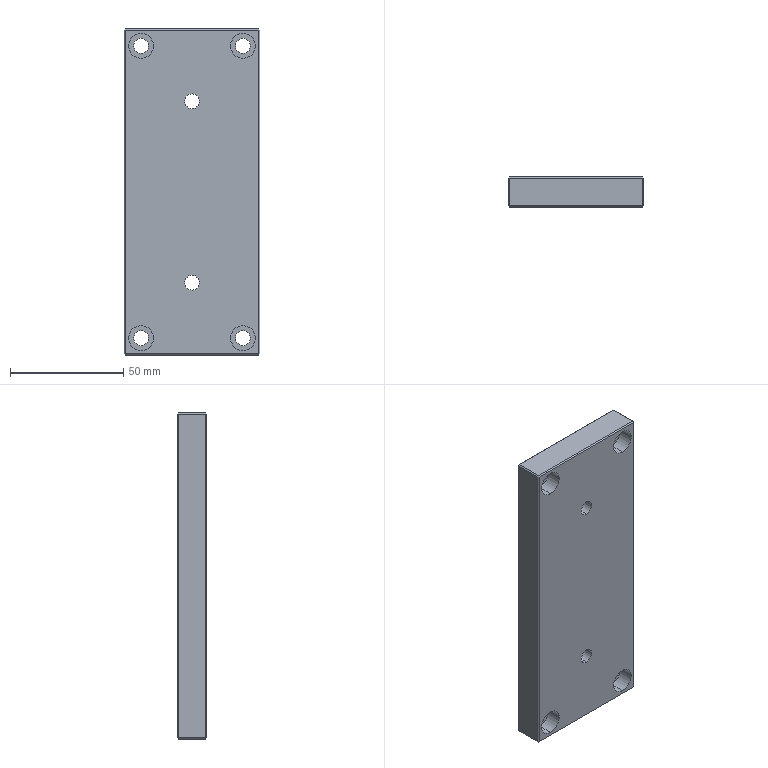Part | SolidWorks | features HoleWzd 2, Chamfer 1, Extrusion 1 | 1 solid | 56 faces | box 60 x 13 x 144 mm | volume 107062 mm3 | plane 32 | cylinder 24 | commonest cylinder face diameters 6.6 x12 11 x12
STEP:
#1=CARTESIAN_POINT('',(22.5,0.3,142.));
#2=VERTEX_POINT('',#1);
#3=CARTESIAN_POINT('',(22.5,0.3,131.));
#4=VERTEX_POINT('',#3);
#5=CARTESIAN_POINT('',(22.5,0.3,136.5));
#6=DIRECTION('',(0.,-1.,0.));
#7=DIRECTION('',(0.,0.,-1.));
#8=AXIS2_PLACEMENT_3D('',#5,#6,#7);
#9=CIRCLE('',#8,5.5);
#10=EDGE_CURVE('',#2,#4,#9,.T.);
#11=ORIENTED_EDGE('',*,*,#10,.F.);
#12=CARTESIAN_POINT('',(22.5,-6.5,142.));
#13=VERTEX_POINT('',#12);
#14=CARTESIAN_POINT('',(22.5,-6.5,142.));
#15=DIRECTION('',(0.,-1.,0.));
#16=VECTOR('',#15,1000.);
#17=LINE('',#14,#16);
#18=EDGE_CURVE('',#2,#13,#17,.T.);
#19=ORIENTED_EDGE('',*,*,#18,.T.);
#20=CARTESIAN_POINT('',(22.5,-6.5,131.));
#21=VERTEX_POINT('',#20);
#22=CARTESIAN_POINT('',(22.5,-6.5,136.5));
#23=DIRECTION('',(0.,-1.,0.));
#24=DIRECTION('',(0.,0.,-1.));
#25=AXIS2_PLACEMENT_3D('',#22,#23,#24);
#26=CIRCLE('',#25,5.5);
#27=EDGE_CURVE('',#13,#21,#26,.T.);
#28=ORIENTED_EDGE('',*,*,#27,.T.);
#29=CARTESIAN_POINT('',(22.5,-6.5,131.));
#30=DIRECTION('',(0.,-1.,0.));
#31=VECTOR('',#30,1000.);
#32=LINE('',#29,#31);
#33=EDGE_CURVE('',#4,#21,#32,.T.);
#34=ORIENTED_EDGE('',*,*,#33,.F.);
#35=EDGE_LOOP('',(#11,#19,#28,#34));
#36=FACE_OUTER_BOUND('',#35,.T.);
#37=CARTESIAN_POINT('',(22.5,-6.5,136.5));
#38=DIRECTION('',(0.,-1.,0.));
#39=DIRECTION('',(0.,0.,-1.));
#40=AXIS2_PLACEMENT_3D('',#37,#38,#39);
#41=CYLINDRICAL_SURFACE('',#40,5.5);
#42=ADVANCED_FACE('',(#36),#41,.F.);
#43=CARTESIAN_POINT('',(22.5,6.5,139.8));
#44=VERTEX_POINT('',#43);
#45=CARTESIAN_POINT('',(22.5,6.5,133.2));
#46=VERTEX_POINT('',#45);
#47=CARTESIAN_POINT('',(22.5,6.5,136.5));
#48=DIRECTION('',(0.,-1.,0.));
#49=DIRECTION('',(0.,0.,-1.));
#50=AXIS2_PLACEMENT_3D('',#47,#48,#49);
#51=CIRCLE('',#50,3.3);
#52=EDGE_CURVE('',#44,#46,#51,.T.);
#53=ORIENTED_EDGE('',*,*,#52,.F.);
#54=CARTESIAN_POINT('',(22.5,0.3,139.8));
#55=VERTEX_POINT('',#54);
#56=CARTESIAN_POINT('',(22.5,-6.5,139.8));
#57=DIRECTION('',(0.,-1.,0.));
#58=VECTOR('',#57,1000.);
#59=LINE('',#56,#58);
#60=EDGE_CURVE('',#44,#55,#59,.T.);
#61=ORIENTED_EDGE('',*,*,#60,.T.);
#62=CARTESIAN_POINT('',(22.5,0.3,133.2));
#63=VERTEX_POINT('',#62);
#64=CARTESIAN_POINT('',(22.5,0.3,136.5));
#65=DIRECTION('',(0.,-1.,0.));
#66=DIRECTION('',(0.,0.,-1.));
#67=AXIS2_PLACEMENT_3D('',#64,#65,#66);
#68=CIRCLE('',#67,3.3);
#69=EDGE_CURVE('',#55,#63,#68,.T.);
#70=ORIENTED_EDGE('',*,*,#69,.T.);
#71=CARTESIAN_POINT('',(22.5,-6.5,133.2));
#72=DIRECTION('',(0.,-1.,0.));
#73=VECTOR('',#72,1000.);
#74=LINE('',#71,#73);
#75=EDGE_CURVE('',#46,#63,#74,.T.);
#76=ORIENTED_EDGE('',*,*,#75,.F.);
#77=EDGE_LOOP('',(#53,#61,#70,#76));
#78=FACE_OUTER_BOUND('',#77,.T.);
#79=CARTESIAN_POINT('',(22.5,-6.5,136.5));
#80=DIRECTION('',(0.,-1.,0.));
#81=DIRECTION('',(0.,0.,-1.));
#82=AXIS2_PLACEMENT_3D('',#79,#80,#81);
#83=CYLINDRICAL_SURFACE('',#82,3.3);
#84=ADVANCED_FACE('',(#78),#83,.F.);
#85=CARTESIAN_POINT('',(-22.5,0.3,142.));
#86=VERTEX_POINT('',#85);
#87=CARTESIAN_POINT('',(-22.5,0.3,131.));
#88=VERTEX_POINT('',#87);
#89=CARTESIAN_POINT('',(-22.5,0.3,136.5));
#90=DIRECTION('',(0.,-1.,0.));
#91=DIRECTION('',(0.,0.,-1.));
#92=AXIS2_PLACEMENT_3D('',#89,#90,#91);
#93=CIRCLE('',#92,5.5);
#94=EDGE_CURVE('',#86,#88,#93,.T.);
#95=ORIENTED_EDGE('',*,*,#94,.F.);
#96=CARTESIAN_POINT('',(-22.5,-6.5,142.));
#97=VERTEX_POINT('',#96);
#98=CARTESIAN_POINT('',(-22.5,-6.5,142.));
#99=DIRECTION('',(0.,-1.,0.));
#100=VECTOR('',#99,1000.);
#101=LINE('',#98,#100);
#102=EDGE_CURVE('',#86,#97,#101,.T.);
#103=ORIENTED_EDGE('',*,*,#102,.T.);
#104=CARTESIAN_POINT('',(-22.5,-6.5,131.));
#105=VERTEX_POINT('',#104);
#106=CARTESIAN_POINT('',(-22.5,-6.5,136.5));
#107=DIRECTION('',(0.,-1.,0.));
#108=DIRECTION('',(0.,0.,-1.));
#109=AXIS2_PLACEMENT_3D('',#106,#107,#108);
#110=CIRCLE('',#109,5.5);
#111=EDGE_CURVE('',#97,#105,#110,.T.);
#112=ORIENTED_EDGE('',*,*,#111,.T.);
#113=CARTESIAN_POINT('',(-22.5,-6.5,131.));
#114=DIRECTION('',(0.,-1.,0.));
#115=VECTOR('',#114,1000.);
#116=LINE('',#113,#115);
#117=EDGE_CURVE('',#88,#105,#116,.T.);
#118=ORIENTED_EDGE('',*,*,#117,.F.);
#119=EDGE_LOOP('',(#95,#103,#112,#118));
#120=FACE_OUTER_BOUND('',#119,.T.);
#121=CARTESIAN_POINT('',(-22.5,-6.5,136.5));
#122=DIRECTION('',(0.,-1.,0.));
#123=DIRECTION('',(0.,0.,-1.));
#124=AXIS2_PLACEMENT_3D('',#121,#122,#123);
#125=CYLINDRICAL_SURFACE('',#124,5.5);
#126=ADVANCED_FACE('',(#120),#125,.F.);
#127=CARTESIAN_POINT('',(-22.5,6.5,139.8));
#128=VERTEX_POINT('',#127);
#129=CARTESIAN_POINT('',(-22.5,6.5,133.2));
#130=VERTEX_POINT('',#129);
#131=CARTESIAN_POINT('',(-22.5,6.5,136.5));
#132=DIRECTION('',(0.,-1.,0.));
#133=DIRECTION('',(0.,0.,-1.));
#134=AXIS2_PLACEMENT_3D('',#131,#132,#133);
#135=CIRCLE('',#134,3.3);
#136=EDGE_CURVE('',#128,#130,#135,.T.);
#137=ORIENTED_EDGE('',*,*,#136,.F.);
#138=CARTESIAN_POINT('',(-22.5,0.3,139.8));
#139=VERTEX_POINT('',#138);
#140=CARTESIAN_POINT('',(-22.5,-6.5,139.8));
#141=DIRECTION('',(0.,-1.,0.));
#142=VECTOR('',#141,1000.);
#143=LINE('',#140,#142);
#144=EDGE_CURVE('',#128,#139,#143,.T.);
#145=ORIENTED_EDGE('',*,*,#144,.T.);
#146=CARTESIAN_POINT('',(-22.5,0.3,133.2));
#147=VERTEX_POINT('',#146);
#148=CARTESIAN_POINT('',(-22.5,0.3,136.5));
#149=DIRECTION('',(0.,-1.,0.));
#150=DIRECTION('',(0.,0.,-1.));
#151=AXIS2_PLACEMENT_3D('',#148,#149,#150);
#152=CIRCLE('',#151,3.3);
#153=EDGE_CURVE('',#139,#147,#152,.T.);
#154=ORIENTED_EDGE('',*,*,#153,.T.);
#155=CARTESIAN_POINT('',(-22.5,-6.5,133.2));
#156=DIRECTION('',(0.,-1.,0.));
#157=VECTOR('',#156,1000.);
#158=LINE('',#155,#157);
#159=EDGE_CURVE('',#130,#147,#158,.T.);
#160=ORIENTED_EDGE('',*,*,#159,.F.);
#161=EDGE_LOOP('',(#137,#145,#154,#160));
#162=FACE_OUTER_BOUND('',#161,.T.);
#163=CARTESIAN_POINT('',(-22.5,-6.5,136.5));
#164=DIRECTION('',(0.,-1.,0.));
#165=DIRECTION('',(0.,0.,-1.));
#166=AXIS2_PLACEMENT_3D('',#163,#164,#165);
#167=CYLINDRICAL_SURFACE('',#166,3.3);
#168=ADVANCED_FACE('',(#162),#167,.F.);
#169=CARTESIAN_POINT('',(22.5,0.3,13.));
#170=VERTEX_POINT('',#169);
#171=CARTESIAN_POINT('',(22.5,0.3,2.));
#172=VERTEX_POINT('',#171);
#173=CARTESIAN_POINT('',(22.5,0.3,7.5));
#174=DIRECTION('',(0.,-1.,0.));
#175=DIRECTION('',(0.,0.,-1.));
#176=AXIS2_PLACEMENT_3D('',#173,#174,#175);
#177=CIRCLE('',#176,5.5);
#178=EDGE_CURVE('',#170,#172,#177,.T.);
#179=ORIENTED_EDGE('',*,*,#178,.F.);
#180=CARTESIAN_POINT('',(22.5,-6.5,13.));
#181=VERTEX_POINT('',#180);
#182=CARTESIAN_POINT('',(22.5,-6.5,13.));
#183=DIRECTION('',(0.,-1.,0.));
#184=VECTOR('',#183,1000.);
#185=LINE('',#182,#184);
#186=EDGE_CURVE('',#170,#181,#185,.T.);
#187=ORIENTED_EDGE('',*,*,#186,.T.);
#188=CARTESIAN_POINT('',(22.5,-6.5,2.));
#189=VERTEX_POINT('',#188);
#190=CARTESIAN_POINT('',(22.5,-6.5,7.5));
#191=DIRECTION('',(0.,-1.,0.));
#192=DIRECTION('',(0.,0.,-1.));
#193=AXIS2_PLACEMENT_3D('',#190,#191,#192);
#194=CIRCLE('',#193,5.5);
#195=EDGE_CURVE('',#181,#189,#194,.T.);
#196=ORIENTED_EDGE('',*,*,#195,.T.);
#197=CARTESIAN_POINT('',(22.5,-6.5,2.));
#198=DIRECTION('',(0.,-1.,0.));
#199=VECTOR('',#198,1000.);
#200=LINE('',#197,#199);
#201=EDGE_CURVE('',#172,#189,#200,.T.);
#202=ORIENTED_EDGE('',*,*,#201,.F.);
#203=EDGE_LOOP('',(#179,#187,#196,#202));
#204=FACE_OUTER_BOUND('',#203,.T.);
#205=CARTESIAN_POINT('',(22.5,-6.5,7.5));
#206=DIRECTION('',(0.,-1.,0.));
#207=DIRECTION('',(0.,0.,-1.));
#208=AXIS2_PLACEMENT_3D('',#205,#206,#207);
#209=CYLINDRICAL_SURFACE('',#208,5.5);
#210=ADVANCED_FACE('',(#204),#209,.F.);
#211=CARTESIAN_POINT('',(22.5,6.5,10.8));
#212=VERTEX_POINT('',#211);
#213=CARTESIAN_POINT('',(22.5,6.5,4.2));
#214=VERTEX_POINT('',#213);
#215=CARTESIAN_POINT('',(22.5,6.5,7.5));
#216=DIRECTION('',(0.,-1.,0.));
#217=DIRECTION('',(0.,0.,-1.));
#218=AXIS2_PLACEMENT_3D('',#215,#216,#217);
#219=CIRCLE('',#218,3.3);
#220=EDGE_CURVE('',#212,#214,#219,.T.);
#221=ORIENTED_EDGE('',*,*,#220,.F.);
#222=CARTESIAN_POINT('',(22.5,0.3,10.8));
#223=VERTEX_POINT('',#222);
#224=CARTESIAN_POINT('',(22.5,-6.5,10.8));
#225=DIRECTION('',(0.,-1.,0.));
#226=VECTOR('',#225,1000.);
#227=LINE('',#224,#226);
#228=EDGE_CURVE('',#212,#223,#227,.T.);
#229=ORIENTED_EDGE('',*,*,#228,.T.);
#230=CARTESIAN_POINT('',(22.5,0.3,4.2));
#231=VERTEX_POINT('',#230);
#232=CARTESIAN_POINT('',(22.5,0.3,7.5));
#233=DIRECTION('',(0.,-1.,0.));
#234=DIRECTION('',(0.,0.,-1.));
#235=AXIS2_PLACEMENT_3D('',#232,#233,#234);
#236=CIRCLE('',#235,3.3);
#237=EDGE_CURVE('',#223,#231,#236,.T.);
#238=ORIENTED_EDGE('',*,*,#237,.T.);
#239=CARTESIAN_POINT('',(22.5,-6.5,4.2));
#240=DIRECTION('',(0.,-1.,0.));
#241=VECTOR('',#240,1000.);
#242=LINE('',#239,#241);
#243=EDGE_CURVE('',#214,#231,#242,.T.);
#244=ORIENTED_EDGE('',*,*,#243,.F.);
#245=EDGE_LOOP('',(#221,#229,#238,#244));
#246=FACE_OUTER_BOUND('',#245,.T.);
#247=CARTESIAN_POINT('',(22.5,-6.5,7.5));
#248=DIRECTION('',(0.,-1.,0.));
#249=DIRECTION('',(0.,0.,-1.));
#250=AXIS2_PLACEMENT_3D('',#247,#248,#249);
#251=CYLINDRICAL_SURFACE('',#250,3.3);
#252=ADVANCED_FACE('',(#246),#251,.F.);
#253=CARTESIAN_POINT('',(-22.5,0.3,13.));
#254=VERTEX_POINT('',#253);
#255=CARTESIAN_POINT('',(-22.5,0.3,2.));
#256=VERTEX_POINT('',#255);
#257=CARTESIAN_POINT('',(-22.5,0.3,7.5));
#258=DIRECTION('',(0.,-1.,0.));
#259=DIRECTION('',(0.,0.,-1.));
#260=AXIS2_PLACEMENT_3D('',#257,#258,#259);
#261=CIRCLE('',#260,5.5);
#262=EDGE_CURVE('',#254,#256,#261,.T.);
#263=ORIENTED_EDGE('',*,*,#262,.F.);
#264=CARTESIAN_POINT('',(-22.5,-6.5,13.));
#265=VERTEX_POINT('',#264);
#266=CARTESIAN_POINT('',(-22.5,-6.5,13.));
#267=DIRECTION('',(0.,-1.,0.));
#268=VECTOR('',#267,1000.);
#269=LINE('',#266,#268);
#270=EDGE_CURVE('',#254,#265,#269,.T.);
#271=ORIENTED_EDGE('',*,*,#270,.T.);
#272=CARTESIAN_POINT('',(-22.5,-6.5,2.));
#273=VERTEX_POINT('',#272);
#274=CARTESIAN_POINT('',(-22.5,-6.5,7.5));
#275=DIRECTION('',(0.,-1.,0.));
#276=DIRECTION('',(0.,0.,-1.));
#277=AXIS2_PLACEMENT_3D('',#274,#275,#276);
#278=CIRCLE('',#277,5.5);
#279=EDGE_CURVE('',#265,#273,#278,.T.);
#280=ORIENTED_EDGE('',*,*,#279,.T.);
#281=CARTESIAN_POINT('',(-22.5,-6.5,2.));
#282=DIRECTION('',(0.,-1.,0.));
#283=VECTOR('',#282,1000.);
#284=LINE('',#281,#283);
#285=EDGE_CURVE('',#256,#273,#284,.T.);
#286=ORIENTED_EDGE('',*,*,#285,.F.);
#287=EDGE_LOOP('',(#263,#271,#280,#286));
#288=FACE_OUTER_BOUND('',#287,.T.);
#289=CARTESIAN_POINT('',(-22.5,-6.5,7.5));
#290=DIRECTION('',(0.,-1.,0.));
#291=DIRECTION('',(0.,0.,-1.));
#292=AXIS2_PLACEMENT_3D('',#289,#290,#291);
#293=CYLINDRICAL_SURFACE('',#292,5.5);
#294=ADVANCED_FACE('',(#288),#293,.F.);
#295=CARTESIAN_POINT('',(-22.5,6.5,10.8));
#296=VERTEX_POINT('',#295);
#297=CARTESIAN_POINT('',(-22.5,6.5,4.2));
#298=VERTEX_POINT('',#297);
#299=CARTESIAN_POINT('',(-22.5,6.5,7.5));
#300=DIRECTION('',(0.,-1.,0.));
#301=DIRECTION('',(0.,0.,-1.));
#302=AXIS2_PLACEMENT_3D('',#299,#300,#301);
#303=CIRCLE('',#302,3.3);
#304=EDGE_CURVE('',#296,#298,#303,.T.);
#305=ORIENTED_EDGE('',*,*,#304,.F.);
#306=CARTESIAN_POINT('',(-22.5,0.3,10.8));
#307=VERTEX_POINT('',#306);
#308=CARTESIAN_POINT('',(-22.5,-6.5,10.8));
#309=DIRECTION('',(0.,-1.,0.));
#310=VECTOR('',#309,1000.);
#311=LINE('',#308,#310);
#312=EDGE_CURVE('',#296,#307,#311,.T.);
#313=ORIENTED_EDGE('',*,*,#312,.T.);
#314=CARTESIAN_POINT('',(-22.5,0.3,4.2));
#315=VERTEX_POINT('',#314);
#316=CARTESIAN_POINT('',(-22.5,0.3,7.5));
#317=DIRECTION('',(0.,-1.,0.));
#318=DIRECTION('',(0.,0.,-1.));
#319=AXIS2_PLACEMENT_3D('',#316,#317,#318);
#320=CIRCLE('',#319,3.3);
#321=EDGE_CURVE('',#307,#315,#320,.T.);
#322=ORIENTED_EDGE('',*,*,#321,.T.);
#323=CARTESIAN_POINT('',(-22.5,-6.5,4.2));
#324=DIRECTION('',(0.,-1.,0.));
#325=VECTOR('',#324,1000.);
#326=LINE('',#323,#325);
#327=EDGE_CURVE('',#298,#315,#326,.T.);
#328=ORIENTED_EDGE('',*,*,#327,.F.);
#329=EDGE_LOOP('',(#305,#313,#322,#328));
#330=FACE_OUTER_BOUND('',#329,.T.);
#331=CARTESIAN_POINT('',(-22.5,-6.5,7.5));
#332=DIRECTION('',(0.,-1.,0.));
#333=DIRECTION('',(0.,0.,-1.));
#334=AXIS2_PLACEMENT_3D('',#331,#332,#333);
#335=CYLINDRICAL_SURFACE('',#334,3.3);
#336=ADVANCED_FACE('',(#330),#335,.F.);
#337=CARTESIAN_POINT('',(0.,-0.3,26.5));
#338=VERTEX_POINT('',#337);
#339=CARTESIAN_POINT('',(0.,-0.3,37.5));
#340=VERTEX_POINT('',#339);
#341=CARTESIAN_POINT('',(0.,-0.3,32.));
#342=DIRECTION('',(0.,1.,0.));
#343=DIRECTION('',(0.,0.,1.));
#344=AXIS2_PLACEMENT_3D('',#341,#342,#343);
#345=CIRCLE('',#344,5.5);
#346=EDGE_CURVE('',#338,#340,#345,.T.);
#347=ORIENTED_EDGE('',*,*,#346,.F.);
#348=CARTESIAN_POINT('',(0.,6.5,26.5));
#349=VERTEX_POINT('',#348);
#350=CARTESIAN_POINT('',(0.,6.5,26.5));
#351=DIRECTION('',(0.,1.,0.));
#352=VECTOR('',#351,1000.);
#353=LINE('',#350,#352);
#354=EDGE_CURVE('',#338,#349,#353,.T.);
#355=ORIENTED_EDGE('',*,*,#354,.T.);
#356=CARTESIAN_POINT('',(0.,6.5,37.5));
#357=VERTEX_POINT('',#356);
#358=CARTESIAN_POINT('',(0.,6.5,32.));
#359=DIRECTION('',(0.,1.,0.));
#360=DIRECTION('',(0.,0.,1.));
#361=AXIS2_PLACEMENT_3D('',#358,#359,#360);
#362=CIRCLE('',#361,5.5);
#363=EDGE_CURVE('',#349,#357,#362,.T.);
#364=ORIENTED_EDGE('',*,*,#363,.T.);
#365=CARTESIAN_POINT('',(0.,6.5,37.5));
#366=DIRECTION('',(0.,1.,0.));
#367=VECTOR('',#366,1000.);
#368=LINE('',#365,#367);
#369=EDGE_CURVE('',#340,#357,#368,.T.);
#370=ORIENTED_EDGE('',*,*,#369,.F.);
#371=EDGE_LOOP('',(#347,#355,#364,#370));
#372=FACE_OUTER_BOUND('',#371,.T.);
#373=CARTESIAN_POINT('',(0.,6.5,32.));
#374=DIRECTION('',(0.,1.,0.));
#375=DIRECTION('',(0.,0.,1.));
#376=AXIS2_PLACEMENT_3D('',#373,#374,#375);
#377=CYLINDRICAL_SURFACE('',#376,5.5);
#378=ADVANCED_FACE('',(#372),#377,.F.);
#379=CARTESIAN_POINT('',(0.,-6.5,28.7));
#380=VERTEX_POINT('',#379);
#381=CARTESIAN_POINT('',(0.,-6.5,35.3));
#382=VERTEX_POINT('',#381);
#383=CARTESIAN_POINT('',(0.,-6.5,32.));
#384=DIRECTION('',(0.,1.,0.));
#385=DIRECTION('',(0.,0.,1.));
#386=AXIS2_PLACEMENT_3D('',#383,#384,#385);
#387=CIRCLE('',#386,3.3);
#388=EDGE_CURVE('',#380,#382,#387,.T.);
#389=ORIENTED_EDGE('',*,*,#388,.F.);
#390=CARTESIAN_POINT('',(0.,-0.3,28.7));
#391=VERTEX_POINT('',#390);
#392=CARTESIAN_POINT('',(0.,6.5,28.7));
#393=DIRECTION('',(0.,1.,0.));
#394=VECTOR('',#393,1000.);
#395=LINE('',#392,#394);
#396=EDGE_CURVE('',#380,#391,#395,.T.);
#397=ORIENTED_EDGE('',*,*,#396,.T.);
#398=CARTESIAN_POINT('',(0.,-0.3,35.3));
#399=VERTEX_POINT('',#398);
#400=CARTESIAN_POINT('',(0.,-0.3,32.));
#401=DIRECTION('',(0.,1.,0.));
#402=DIRECTION('',(0.,0.,1.));
#403=AXIS2_PLACEMENT_3D('',#400,#401,#402);
#404=CIRCLE('',#403,3.3);
#405=EDGE_CURVE('',#391,#399,#404,.T.);
#406=ORIENTED_EDGE('',*,*,#405,.T.);
#407=CARTESIAN_POINT('',(0.,6.5,35.3));
#408=DIRECTION('',(0.,1.,0.));
#409=VECTOR('',#408,1000.);
#410=LINE('',#407,#409);
#411=EDGE_CURVE('',#382,#399,#410,.T.);
#412=ORIENTED_EDGE('',*,*,#411,.F.);
#413=EDGE_LOOP('',(#389,#397,#406,#412));
#414=FACE_OUTER_BOUND('',#413,.T.);
#415=CARTESIAN_POINT('',(0.,6.5,32.));
#416=DIRECTION('',(0.,1.,0.));
#417=DIRECTION('',(0.,0.,1.));
#418=AXIS2_PLACEMENT_3D('',#415,#416,#417);
#419=CYLINDRICAL_SURFACE('',#418,3.3);
#420=ADVANCED_FACE('',(#414),#419,.F.);
#421=CARTESIAN_POINT('',(0.,-0.3,106.5));
#422=VERTEX_POINT('',#421);
#423=CARTESIAN_POINT('',(0.,-0.3,117.5));
#424=VERTEX_POINT('',#423);
#425=CARTESIAN_POINT('',(0.,-0.3,112.));
#426=DIRECTION('',(0.,1.,0.));
#427=DIRECTION('',(0.,0.,1.));
#428=AXIS2_PLACEMENT_3D('',#425,#426,#427);
#429=CIRCLE('',#428,5.5);
#430=EDGE_CURVE('',#422,#424,#429,.T.);
#431=ORIENTED_EDGE('',*,*,#430,.F.);
#432=CARTESIAN_POINT('',(0.,6.5,106.5));
#433=VERTEX_POINT('',#432);
#434=CARTESIAN_POINT('',(0.,6.5,106.5));
#435=DIRECTION('',(0.,1.,0.));
#436=VECTOR('',#435,1000.);
#437=LINE('',#434,#436);
#438=EDGE_CURVE('',#422,#433,#437,.T.);
#439=ORIENTED_EDGE('',*,*,#438,.T.);
#440=CARTESIAN_POINT('',(0.,6.5,117.5));
#441=VERTEX_POINT('',#440);
#442=CARTESIAN_POINT('',(0.,6.5,112.));
#443=DIRECTION('',(0.,1.,0.));
#444=DIRECTION('',(0.,0.,1.));
#445=AXIS2_PLACEMENT_3D('',#442,#443,#444);
#446=CIRCLE('',#445,5.5);
#447=EDGE_CURVE('',#433,#441,#446,.T.);
#448=ORIENTED_EDGE('',*,*,#447,.T.);
#449=CARTESIAN_POINT('',(0.,6.5,117.5));
#450=DIRECTION('',(0.,1.,0.));
#451=VECTOR('',#450,1000.);
#452=LINE('',#449,#451);
#453=EDGE_CURVE('',#424,#441,#452,.T.);
#454=ORIENTED_EDGE('',*,*,#453,.F.);
#455=EDGE_LOOP('',(#431,#439,#448,#454));
#456=FACE_OUTER_BOUND('',#455,.T.);
#457=CARTESIAN_POINT('',(0.,6.5,112.));
#458=DIRECTION('',(0.,1.,0.));
#459=DIRECTION('',(0.,0.,1.));
#460=AXIS2_PLACEMENT_3D('',#457,#458,#459);
#461=CYLINDRICAL_SURFACE('',#460,5.5);
#462=ADVANCED_FACE('',(#456),#461,.F.);
#463=CARTESIAN_POINT('',(0.,-6.5,108.7));
#464=VERTEX_POINT('',#463);
#465=CARTESIAN_POINT('',(0.,-6.5,115.3));
#466=VERTEX_POINT('',#465);
#467=CARTESIAN_POINT('',(0.,-6.5,112.));
#468=DIRECTION('',(0.,1.,0.));
#469=DIRECTION('',(0.,0.,1.));
#470=AXIS2_PLACEMENT_3D('',#467,#468,#469);
#471=CIRCLE('',#470,3.3);
#472=EDGE_CURVE('',#464,#466,#471,.T.);
#473=ORIENTED_EDGE('',*,*,#472,.F.);
#474=CARTESIAN_POINT('',(0.,-0.3,108.7));
#475=VERTEX_POINT('',#474);
#476=CARTESIAN_POINT('',(0.,6.5,108.7));
#477=DIRECTION('',(0.,1.,0.));
#478=VECTOR('',#477,1000.);
#479=LINE('',#476,#478);
#480=EDGE_CURVE('',#464,#475,#479,.T.);
#481=ORIENTED_EDGE('',*,*,#480,.T.);
#482=CARTESIAN_POINT('',(0.,-0.3,115.3));
#483=VERTEX_POINT('',#482);
#484=CARTESIAN_POINT('',(0.,-0.3,112.));
#485=DIRECTION('',(0.,1.,0.));
#486=DIRECTION('',(0.,0.,1.));
#487=AXIS2_PLACEMENT_3D('',#484,#485,#486);
#488=CIRCLE('',#487,3.3);
#489=EDGE_CURVE('',#475,#483,#488,.T.);
#490=ORIENTED_EDGE('',*,*,#489,.T.);
#491=CARTESIAN_POINT('',(0.,6.5,115.3));
#492=DIRECTION('',(0.,1.,0.));
#493=VECTOR('',#492,1000.);
#494=LINE('',#491,#493);
#495=EDGE_CURVE('',#466,#483,#494,.T.);
#496=ORIENTED_EDGE('',*,*,#495,.F.);
#497=EDGE_LOOP('',(#473,#481,#490,#496));
#498=FACE_OUTER_BOUND('',#497,.T.);
#499=CARTESIAN_POINT('',(0.,6.5,112.));
#500=DIRECTION('',(0.,1.,0.));
#501=DIRECTION('',(0.,0.,1.));
#502=AXIS2_PLACEMENT_3D('',#499,#500,#501);
#503=CYLINDRICAL_SURFACE('',#502,3.3);
#504=ADVANCED_FACE('',(#498),#503,.F.);
#505=CARTESIAN_POINT('',(30.,6.,143.5));
#506=VERTEX_POINT('',#505);
#507=CARTESIAN_POINT('',(30.,-6.,143.5));
#508=VERTEX_POINT('',#507);
#509=CARTESIAN_POINT('',(30.,-6.5,143.5));
#510=DIRECTION('',(0.,-1.,0.));
#511=VECTOR('',#510,1000.);
#512=LINE('',#509,#511);
#513=EDGE_CURVE('',#506,#508,#512,.T.);
#514=ORIENTED_EDGE('',*,*,#513,.T.);
#515=CARTESIAN_POINT('',(30.,-6.,0.5));
#516=VERTEX_POINT('',#515);
#517=CARTESIAN_POINT('',(30.,-6.,144.));
#518=DIRECTION('',(0.,0.,-1.));
#519=VECTOR('',#518,1000.);
#520=LINE('',#517,#519);
#521=EDGE_CURVE('',#508,#516,#520,.T.);
#522=ORIENTED_EDGE('',*,*,#521,.T.);
#523=CARTESIAN_POINT('',(30.,6.,0.5));
#524=VERTEX_POINT('',#523);
#525=CARTESIAN_POINT('',(30.,6.5,0.5));
#526=DIRECTION('',(0.,1.,0.));
#527=VECTOR('',#526,1000.);
#528=LINE('',#525,#527);
#529=EDGE_CURVE('',#516,#524,#528,.T.);
#530=ORIENTED_EDGE('',*,*,#529,.T.);
#531=CARTESIAN_POINT('',(30.,6.,144.));
#532=DIRECTION('',(0.,0.,1.));
#533=VECTOR('',#532,1000.);
#534=LINE('',#531,#533);
#535=EDGE_CURVE('',#524,#506,#534,.T.);
#536=ORIENTED_EDGE('',*,*,#535,.T.);
#537=EDGE_LOOP('',(#514,#522,#530,#536));
#538=FACE_OUTER_BOUND('',#537,.T.);
#539=CARTESIAN_POINT('',(30.,6.5,144.));
#540=DIRECTION('',(-1.,0.,0.));
#541=DIRECTION('',(0.,0.,1.));
#542=AXIS2_PLACEMENT_3D('',#539,#540,#541);
#543=PLANE('',#542);
#544=ADVANCED_FACE('',(#538),#543,.F.);
#545=CARTESIAN_POINT('',(22.5,6.5,136.5));
#546=DIRECTION('',(0.,-1.,0.));
#547=DIRECTION('',(0.,0.,-1.));
#548=AXIS2_PLACEMENT_3D('',#545,#546,#547);
#549=CIRCLE('',#548,3.3);
#550=EDGE_CURVE('',#46,#44,#549,.T.);
#551=ORIENTED_EDGE('',*,*,#550,.T.);
#552=ORIENTED_EDGE('',*,*,#52,.T.);
#553=EDGE_LOOP('',(#551,#552));
#554=FACE_BOUND('',#553,.T.);
#555=CARTESIAN_POINT('',(-22.5,6.5,136.5));
#556=DIRECTION('',(0.,-1.,0.));
#557=DIRECTION('',(0.,0.,-1.));
#558=AXIS2_PLACEMENT_3D('',#555,#556,#557);
#559=CIRCLE('',#558,3.3);
#560=EDGE_CURVE('',#130,#128,#559,.T.);
#561=ORIENTED_EDGE('',*,*,#560,.T.);
#562=ORIENTED_EDGE('',*,*,#136,.T.);
#563=EDGE_LOOP('',(#561,#562));
#564=FACE_BOUND('',#563,.T.);
#565=CARTESIAN_POINT('',(22.5,6.5,7.5));
#566=DIRECTION('',(0.,-1.,0.));
#567=DIRECTION('',(0.,0.,-1.));
#568=AXIS2_PLACEMENT_3D('',#565,#566,#567);
#569=CIRCLE('',#568,3.3);
#570=EDGE_CURVE('',#214,#212,#569,.T.);
#571=ORIENTED_EDGE('',*,*,#570,.T.);
#572=ORIENTED_EDGE('',*,*,#220,.T.);
#573=EDGE_LOOP('',(#571,#572));
#574=FACE_BOUND('',#573,.T.);
#575=CARTESIAN_POINT('',(-22.5,6.5,7.5));
#576=DIRECTION('',(0.,-1.,0.));
#577=DIRECTION('',(0.,0.,-1.));
#578=AXIS2_PLACEMENT_3D('',#575,#576,#577);
#579=CIRCLE('',#578,3.3);
#580=EDGE_CURVE('',#298,#296,#579,.T.);
#581=ORIENTED_EDGE('',*,*,#580,.T.);
#582=ORIENTED_EDGE('',*,*,#304,.T.);
#583=EDGE_LOOP('',(#581,#582));
#584=FACE_BOUND('',#583,.T.);
#585=CARTESIAN_POINT('',(-29.5,6.5,0.5));
#586=VERTEX_POINT('',#585);
#587=CARTESIAN_POINT('',(-29.5,6.5,143.5));
#588=VERTEX_POINT('',#587);
#589=CARTESIAN_POINT('',(-29.5,6.5,144.));
#590=DIRECTION('',(0.,0.,1.));
#591=VECTOR('',#590,1000.);
#592=LINE('',#589,#591);
#593=EDGE_CURVE('',#586,#588,#592,.T.);
#594=ORIENTED_EDGE('',*,*,#593,.T.);
#595=CARTESIAN_POINT('',(29.5,6.5,143.5));
#596=VERTEX_POINT('',#595);
#597=CARTESIAN_POINT('',(30.,6.5,143.5));
#598=DIRECTION('',(1.,0.,0.));
#599=VECTOR('',#598,1000.);
#600=LINE('',#597,#599);
#601=EDGE_CURVE('',#588,#596,#600,.T.);
#602=ORIENTED_EDGE('',*,*,#601,.T.);
#603=CARTESIAN_POINT('',(29.5,6.5,0.5));
#604=VERTEX_POINT('',#603);
#605=CARTESIAN_POINT('',(29.5,6.5,144.));
#606=DIRECTION('',(0.,0.,-1.));
#607=VECTOR('',#606,1000.);
#608=LINE('',#605,#607);
#609=EDGE_CURVE('',#596,#604,#608,.T.);
#610=ORIENTED_EDGE('',*,*,#609,.T.);
#611=CARTESIAN_POINT('',(-30.,6.5,0.5));
#612=DIRECTION('',(-1.,0.,0.));
#613=VECTOR('',#612,1000.);
#614=LINE('',#611,#613);
#615=EDGE_CURVE('',#604,#586,#614,.T.);
#616=ORIENTED_EDGE('',*,*,#615,.T.);
#617=EDGE_LOOP('',(#594,#602,#610,#616));
#618=FACE_OUTER_BOUND('',#617,.T.);
#619=CARTESIAN_POINT('',(0.,6.5,32.));
#620=DIRECTION('',(0.,1.,0.));
#621=DIRECTION('',(0.,0.,1.));
#622=AXIS2_PLACEMENT_3D('',#619,#620,#621);
#623=CIRCLE('',#622,5.5);
#624=EDGE_CURVE('',#357,#349,#623,.T.);
#625=ORIENTED_EDGE('',*,*,#624,.F.);
#626=ORIENTED_EDGE('',*,*,#363,.F.);
#627=EDGE_LOOP('',(#625,#626));
#628=FACE_BOUND('',#627,.T.);
#629=CARTESIAN_POINT('',(0.,6.5,112.));
#630=DIRECTION('',(0.,1.,0.));
#631=DIRECTION('',(0.,0.,1.));
#632=AXIS2_PLACEMENT_3D('',#629,#630,#631);
#633=CIRCLE('',#632,5.5);
#634=EDGE_CURVE('',#441,#433,#633,.T.);
#635=ORIENTED_EDGE('',*,*,#634,.F.);
#636=ORIENTED_EDGE('',*,*,#447,.F.);
#637=EDGE_LOOP('',(#635,#636));
#638=FACE_BOUND('',#637,.T.);
#639=CARTESIAN_POINT('',(-30.,6.5,144.));
#640=DIRECTION('',(0.,-1.,0.));
#641=DIRECTION('',(0.,0.,-1.));
#642=AXIS2_PLACEMENT_3D('',#639,#640,#641);
#643=PLANE('',#642);
#644=ADVANCED_FACE('',(#554,#564,#574,#584,#618,#628,#638),#643,.F.);
#645=CARTESIAN_POINT('',(-30.,-6.,143.5));
#646=VERTEX_POINT('',#645);
#647=CARTESIAN_POINT('',(-30.,6.,143.5));
#648=VERTEX_POINT('',#647);
#649=CARTESIAN_POINT('',(-30.,6.5,143.5));
#650=DIRECTION('',(0.,1.,0.));
#651=VECTOR('',#650,1000.);
#652=LINE('',#649,#651);
#653=EDGE_CURVE('',#646,#648,#652,.T.);
#654=ORIENTED_EDGE('',*,*,#653,.T.);
#655=CARTESIAN_POINT('',(-30.,6.,0.5));
#656=VERTEX_POINT('',#655);
#657=CARTESIAN_POINT('',(-30.,6.,144.));
#658=DIRECTION('',(0.,0.,-1.));
#659=VECTOR('',#658,1000.);
#660=LINE('',#657,#659);
#661=EDGE_CURVE('',#648,#656,#660,.T.);
#662=ORIENTED_EDGE('',*,*,#661,.T.);
#663=CARTESIAN_POINT('',(-30.,-6.,0.5));
#664=VERTEX_POINT('',#663);
#665=CARTESIAN_POINT('',(-30.,6.5,0.5));
#666=DIRECTION('',(0.,-1.,0.));
#667=VECTOR('',#666,1000.);
#668=LINE('',#665,#667);
#669=EDGE_CURVE('',#656,#664,#668,.T.);
#670=ORIENTED_EDGE('',*,*,#669,.T.);
#671=CARTESIAN_POINT('',(-30.,-6.,144.));
#672=DIRECTION('',(0.,0.,1.));
#673=VECTOR('',#672,1000.);
#674=LINE('',#671,#673);
#675=EDGE_CURVE('',#664,#646,#674,.T.);
#676=ORIENTED_EDGE('',*,*,#675,.T.);
#677=EDGE_LOOP('',(#654,#662,#670,#676));
#678=FACE_OUTER_BOUND('',#677,.T.);
#679=CARTESIAN_POINT('',(-30.,6.5,144.));
#680=DIRECTION('',(1.,0.,0.));
#681=DIRECTION('',(0.,0.,-1.));
#682=AXIS2_PLACEMENT_3D('',#679,#680,#681);
#683=PLANE('',#682);
#684=ADVANCED_FACE('',(#678),#683,.F.);
#685=CARTESIAN_POINT('',(22.5,-6.5,136.5));
#686=DIRECTION('',(0.,-1.,0.));
#687=DIRECTION('',(0.,0.,-1.));
#688=AXIS2_PLACEMENT_3D('',#685,#686,#687);
#689=CIRCLE('',#688,5.5);
#690=EDGE_CURVE('',#21,#13,#689,.T.);
#691=ORIENTED_EDGE('',*,*,#690,.F.);
#692=ORIENTED_EDGE('',*,*,#27,.F.);
#693=EDGE_LOOP('',(#691,#692));
#694=FACE_BOUND('',#693,.T.);
#695=CARTESIAN_POINT('',(-22.5,-6.5,136.5));
#696=DIRECTION('',(0.,-1.,0.));
#697=DIRECTION('',(0.,0.,-1.));
#698=AXIS2_PLACEMENT_3D('',#695,#696,#697);
#699=CIRCLE('',#698,5.5);
#700=EDGE_CURVE('',#105,#97,#699,.T.);
#701=ORIENTED_EDGE('',*,*,#700,.F.);
#702=ORIENTED_EDGE('',*,*,#111,.F.);
#703=EDGE_LOOP('',(#701,#702));
#704=FACE_BOUND('',#703,.T.);
#705=CARTESIAN_POINT('',(22.5,-6.5,7.5));
#706=DIRECTION('',(0.,-1.,0.));
#707=DIRECTION('',(0.,0.,-1.));
#708=AXIS2_PLACEMENT_3D('',#705,#706,#707);
#709=CIRCLE('',#708,5.5);
#710=EDGE_CURVE('',#189,#181,#709,.T.);
#711=ORIENTED_EDGE('',*,*,#710,.F.);
#712=ORIENTED_EDGE('',*,*,#195,.F.);
#713=EDGE_LOOP('',(#711,#712));
#714=FACE_BOUND('',#713,.T.);
#715=CARTESIAN_POINT('',(-22.5,-6.5,7.5));
#716=DIRECTION('',(0.,-1.,0.));
#717=DIRECTION('',(0.,0.,-1.));
#718=AXIS2_PLACEMENT_3D('',#715,#716,#717);
#719=CIRCLE('',#718,5.5);
#720=EDGE_CURVE('',#273,#265,#719,.T.);
#721=ORIENTED_EDGE('',*,*,#720,.F.);
#722=ORIENTED_EDGE('',*,*,#279,.F.);
#723=EDGE_LOOP('',(#721,#722));
#724=FACE_BOUND('',#723,.T.);
#725=CARTESIAN_POINT('',(29.5,-6.5,0.5));
#726=VERTEX_POINT('',#725);
#727=CARTESIAN_POINT('',(29.5,-6.5,143.5));
#728=VERTEX_POINT('',#727);
#729=CARTESIAN_POINT('',(29.5,-6.5,144.));
#730=DIRECTION('',(0.,0.,1.));
#731=VECTOR('',#730,1000.);
#732=LINE('',#729,#731);
#733=EDGE_CURVE('',#726,#728,#732,.T.);
#734=ORIENTED_EDGE('',*,*,#733,.T.);
#735=CARTESIAN_POINT('',(-29.5,-6.5,143.5));
#736=VERTEX_POINT('',#735);
#737=CARTESIAN_POINT('',(-30.,-6.5,143.5));
#738=DIRECTION('',(-1.,0.,0.));
#739=VECTOR('',#738,1000.);
#740=LINE('',#737,#739);
#741=EDGE_CURVE('',#728,#736,#740,.T.);
#742=ORIENTED_EDGE('',*,*,#741,.T.);
#743=CARTESIAN_POINT('',(-29.5,-6.5,0.5));
#744=VERTEX_POINT('',#743);
#745=CARTESIAN_POINT('',(-29.5,-6.5,144.));
#746=DIRECTION('',(0.,0.,-1.));
#747=VECTOR('',#746,1000.);
#748=LINE('',#745,#747);
#749=EDGE_CURVE('',#736,#744,#748,.T.);
#750=ORIENTED_EDGE('',*,*,#749,.T.);
#751=CARTESIAN_POINT('',(-30.,-6.5,0.5));
#752=DIRECTION('',(1.,0.,0.));
#753=VECTOR('',#752,1000.);
#754=LINE('',#751,#753);
#755=EDGE_CURVE('',#744,#726,#754,.T.);
#756=ORIENTED_EDGE('',*,*,#755,.T.);
#757=EDGE_LOOP('',(#734,#742,#750,#756));
#758=FACE_OUTER_BOUND('',#757,.T.);
#759=CARTESIAN_POINT('',(0.,-6.5,32.));
#760=DIRECTION('',(0.,1.,0.));
#761=DIRECTION('',(0.,0.,1.));
#762=AXIS2_PLACEMENT_3D('',#759,#760,#761);
#763=CIRCLE('',#762,3.3);
#764=EDGE_CURVE('',#382,#380,#763,.T.);
#765=ORIENTED_EDGE('',*,*,#764,.T.);
#766=ORIENTED_EDGE('',*,*,#388,.T.);
#767=EDGE_LOOP('',(#765,#766));
#768=FACE_BOUND('',#767,.T.);
#769=CARTESIAN_POINT('',(0.,-6.5,112.));
#770=DIRECTION('',(0.,1.,0.));
#771=DIRECTION('',(0.,0.,1.));
#772=AXIS2_PLACEMENT_3D('',#769,#770,#771);
#773=CIRCLE('',#772,3.3);
#774=EDGE_CURVE('',#466,#464,#773,.T.);
#775=ORIENTED_EDGE('',*,*,#774,.T.);
#776=ORIENTED_EDGE('',*,*,#472,.T.);
#777=EDGE_LOOP('',(#775,#776));
#778=FACE_BOUND('',#777,.T.);
#779=CARTESIAN_POINT('',(-30.,-6.5,144.));
#780=DIRECTION('',(0.,1.,0.));
#781=DIRECTION('',(0.,0.,1.));
#782=AXIS2_PLACEMENT_3D('',#779,#780,#781);
#783=PLANE('',#782);
#784=ADVANCED_FACE('',(#694,#704,#714,#724,#758,#768,#778),#783,.F.);
#785=CARTESIAN_POINT('',(29.5,6.,144.));
#786=VERTEX_POINT('',#785);
#787=CARTESIAN_POINT('',(-29.5,6.,144.));
#788=VERTEX_POINT('',#787);
#789=CARTESIAN_POINT('',(-30.,6.,144.));
#790=DIRECTION('',(-1.,0.,0.));
#791=VECTOR('',#790,1000.);
#792=LINE('',#789,#791);
#793=EDGE_CURVE('',#786,#788,#792,.T.);
#794=ORIENTED_EDGE('',*,*,#793,.T.);
#795=CARTESIAN_POINT('',(-29.5,-6.,144.));
#796=VERTEX_POINT('',#795);
#797=CARTESIAN_POINT('',(-29.5,-6.5,144.));
#798=DIRECTION('',(0.,-1.,0.));
#799=VECTOR('',#798,1000.);
#800=LINE('',#797,#799);
#801=EDGE_CURVE('',#788,#796,#800,.T.);
#802=ORIENTED_EDGE('',*,*,#801,.T.);
#803=CARTESIAN_POINT('',(29.5,-6.,144.));
#804=VERTEX_POINT('',#803);
#805=CARTESIAN_POINT('',(30.,-6.,144.));
#806=DIRECTION('',(1.,0.,0.));
#807=VECTOR('',#806,1000.);
#808=LINE('',#805,#807);
#809=EDGE_CURVE('',#796,#804,#808,.T.);
#810=ORIENTED_EDGE('',*,*,#809,.T.);
#811=CARTESIAN_POINT('',(29.5,6.5,144.));
#812=DIRECTION('',(0.,1.,0.));
#813=VECTOR('',#812,1000.);
#814=LINE('',#811,#813);
#815=EDGE_CURVE('',#804,#786,#814,.T.);
#816=ORIENTED_EDGE('',*,*,#815,.T.);
#817=EDGE_LOOP('',(#794,#802,#810,#816));
#818=FACE_OUTER_BOUND('',#817,.T.);
#819=CARTESIAN_POINT('',(0.,0.,144.));
#820=DIRECTION('',(0.,0.,1.));
#821=DIRECTION('',(1.,0.,0.));
#822=AXIS2_PLACEMENT_3D('',#819,#820,#821);
#823=PLANE('',#822);
#824=ADVANCED_FACE('',(#818),#823,.T.);
#825=CARTESIAN_POINT('',(29.5,-6.,0.));
#826=VERTEX_POINT('',#825);
#827=CARTESIAN_POINT('',(-29.5,-6.,0.));
#828=VERTEX_POINT('',#827);
#829=CARTESIAN_POINT('',(0.,-6.,0.));
#830=DIRECTION('',(-1.,0.,0.));
#831=VECTOR('',#830,1000.);
#832=LINE('',#829,#831);
#833=EDGE_CURVE('',#826,#828,#832,.T.);
#834=ORIENTED_EDGE('',*,*,#833,.T.);
#835=CARTESIAN_POINT('',(-29.5,6.,0.));
#836=VERTEX_POINT('',#835);
#837=CARTESIAN_POINT('',(-29.5,0.,0.));
#838=DIRECTION('',(0.,1.,0.));
#839=VECTOR('',#838,1000.);
#840=LINE('',#837,#839);
#841=EDGE_CURVE('',#828,#836,#840,.T.);
#842=ORIENTED_EDGE('',*,*,#841,.T.);
#843=CARTESIAN_POINT('',(29.5,6.,0.));
#844=VERTEX_POINT('',#843);
#845=CARTESIAN_POINT('',(0.,6.,0.));
#846=DIRECTION('',(1.,0.,0.));
#847=VECTOR('',#846,1000.);
#848=LINE('',#845,#847);
#849=EDGE_CURVE('',#836,#844,#848,.T.);
#850=ORIENTED_EDGE('',*,*,#849,.T.);
#851=CARTESIAN_POINT('',(29.5,0.,0.));
#852=DIRECTION('',(0.,-1.,0.));
#853=VECTOR('',#852,1000.);
#854=LINE('',#851,#853);
#855=EDGE_CURVE('',#844,#826,#854,.T.);
#856=ORIENTED_EDGE('',*,*,#855,.T.);
#857=EDGE_LOOP('',(#834,#842,#850,#856));
#858=FACE_OUTER_BOUND('',#857,.T.);
#859=CARTESIAN_POINT('',(0.,0.,0.));
#860=DIRECTION('',(0.,0.,1.));
#861=DIRECTION('',(1.,0.,0.));
#862=AXIS2_PLACEMENT_3D('',#859,#860,#861);
#863=PLANE('',#862);
#864=ADVANCED_FACE('',(#858),#863,.F.);
#865=ORIENTED_EDGE('',*,*,#480,.F.);
#866=ORIENTED_EDGE('',*,*,#774,.F.);
#867=ORIENTED_EDGE('',*,*,#495,.T.);
#868=CARTESIAN_POINT('',(0.,-0.3,112.));
#869=DIRECTION('',(0.,1.,0.));
#870=DIRECTION('',(0.,0.,1.));
#871=AXIS2_PLACEMENT_3D('',#868,#869,#870);
#872=CIRCLE('',#871,3.3);
#873=EDGE_CURVE('',#483,#475,#872,.T.);
#874=ORIENTED_EDGE('',*,*,#873,.T.);
#875=EDGE_LOOP('',(#865,#866,#867,#874));
#876=FACE_OUTER_BOUND('',#875,.T.);
#877=CARTESIAN_POINT('',(0.,6.5,112.));
#878=DIRECTION('',(0.,1.,0.));
#879=DIRECTION('',(0.,0.,1.));
#880=AXIS2_PLACEMENT_3D('',#877,#878,#879);
#881=CYLINDRICAL_SURFACE('',#880,3.3);
#882=ADVANCED_FACE('',(#876),#881,.F.);
#883=ORIENTED_EDGE('',*,*,#873,.F.);
#884=ORIENTED_EDGE('',*,*,#489,.F.);
#885=EDGE_LOOP('',(#883,#884));
#886=FACE_BOUND('',#885,.T.);
#887=CARTESIAN_POINT('',(0.,-0.3,112.));
#888=DIRECTION('',(0.,1.,0.));
#889=DIRECTION('',(0.,0.,1.));
#890=AXIS2_PLACEMENT_3D('',#887,#888,#889);
#891=CIRCLE('',#890,5.5);
#892=EDGE_CURVE('',#424,#422,#891,.T.);
#893=ORIENTED_EDGE('',*,*,#892,.T.);
#894=ORIENTED_EDGE('',*,*,#430,.T.);
#895=EDGE_LOOP('',(#893,#894));
#896=FACE_OUTER_BOUND('',#895,.T.);
#897=CARTESIAN_POINT('',(3.3,-0.3,112.));
#898=DIRECTION('',(0.,-1.,0.));
#899=DIRECTION('',(0.,0.,-1.));
#900=AXIS2_PLACEMENT_3D('',#897,#898,#899);
#901=PLANE('',#900);
#902=ADVANCED_FACE('',(#886,#896),#901,.F.);
#903=ORIENTED_EDGE('',*,*,#438,.F.);
#904=ORIENTED_EDGE('',*,*,#892,.F.);
#905=ORIENTED_EDGE('',*,*,#453,.T.);
#906=ORIENTED_EDGE('',*,*,#634,.T.);
#907=EDGE_LOOP('',(#903,#904,#905,#906));
#908=FACE_OUTER_BOUND('',#907,.T.);
#909=CARTESIAN_POINT('',(0.,6.5,112.));
#910=DIRECTION('',(0.,1.,0.));
#911=DIRECTION('',(0.,0.,1.));
#912=AXIS2_PLACEMENT_3D('',#909,#910,#911);
#913=CYLINDRICAL_SURFACE('',#912,5.5);
#914=ADVANCED_FACE('',(#908),#913,.F.);
#915=ORIENTED_EDGE('',*,*,#396,.F.);
#916=ORIENTED_EDGE('',*,*,#764,.F.);
#917=ORIENTED_EDGE('',*,*,#411,.T.);
#918=CARTESIAN_POINT('',(0.,-0.3,32.));
#919=DIRECTION('',(0.,1.,0.));
#920=DIRECTION('',(0.,0.,1.));
#921=AXIS2_PLACEMENT_3D('',#918,#919,#920);
#922=CIRCLE('',#921,3.3);
#923=EDGE_CURVE('',#399,#391,#922,.T.);
#924=ORIENTED_EDGE('',*,*,#923,.T.);
#925=EDGE_LOOP('',(#915,#916,#917,#924));
#926=FACE_OUTER_BOUND('',#925,.T.);
#927=CARTESIAN_POINT('',(0.,6.5,32.));
#928=DIRECTION('',(0.,1.,0.));
#929=DIRECTION('',(0.,0.,1.));
#930=AXIS2_PLACEMENT_3D('',#927,#928,#929);
#931=CYLINDRICAL_SURFACE('',#930,3.3);
#932=ADVANCED_FACE('',(#926),#931,.F.);
#933=ORIENTED_EDGE('',*,*,#923,.F.);
#934=ORIENTED_EDGE('',*,*,#405,.F.);
#935=EDGE_LOOP('',(#933,#934));
#936=FACE_BOUND('',#935,.T.);
#937=CARTESIAN_POINT('',(0.,-0.3,32.));
#938=DIRECTION('',(0.,1.,0.));
#939=DIRECTION('',(0.,0.,1.));
#940=AXIS2_PLACEMENT_3D('',#937,#938,#939);
#941=CIRCLE('',#940,5.5);
#942=EDGE_CURVE('',#340,#338,#941,.T.);
#943=ORIENTED_EDGE('',*,*,#942,.T.);
#944=ORIENTED_EDGE('',*,*,#346,.T.);
#945=EDGE_LOOP('',(#943,#944));
#946=FACE_OUTER_BOUND('',#945,.T.);
#947=CARTESIAN_POINT('',(3.3,-0.3,32.));
#948=DIRECTION('',(0.,-1.,0.));
#949=DIRECTION('',(0.,0.,-1.));
#950=AXIS2_PLACEMENT_3D('',#947,#948,#949);
#951=PLANE('',#950);
#952=ADVANCED_FACE('',(#936,#946),#951,.F.);
#953=ORIENTED_EDGE('',*,*,#354,.F.);
#954=ORIENTED_EDGE('',*,*,#942,.F.);
#955=ORIENTED_EDGE('',*,*,#369,.T.);
#956=ORIENTED_EDGE('',*,*,#624,.T.);
#957=EDGE_LOOP('',(#953,#954,#955,#956));
#958=FACE_OUTER_BOUND('',#957,.T.);
#959=CARTESIAN_POINT('',(0.,6.5,32.));
#960=DIRECTION('',(0.,1.,0.));
#961=DIRECTION('',(0.,0.,1.));
#962=AXIS2_PLACEMENT_3D('',#959,#960,#961);
#963=CYLINDRICAL_SURFACE('',#962,5.5);
#964=ADVANCED_FACE('',(#958),#963,.F.);
#965=CARTESIAN_POINT('',(-29.5,6.25,0.25));
#966=DIRECTION('',(0.,-0.7071,-0.7071));
#967=VECTOR('',#966,1000.);
#968=LINE('',#965,#967);
#969=EDGE_CURVE('',#586,#836,#968,.T.);
#970=ORIENTED_EDGE('',*,*,#969,.F.);
#971=ORIENTED_EDGE('',*,*,#615,.F.);
#972=CARTESIAN_POINT('',(29.5,6.5,0.5));
#973=DIRECTION('',(0.,0.7071,0.7071));
#974=VECTOR('',#973,1000.);
#975=LINE('',#972,#974);
#976=EDGE_CURVE('',#844,#604,#975,.T.);
#977=ORIENTED_EDGE('',*,*,#976,.F.);
#978=ORIENTED_EDGE('',*,*,#849,.F.);
#979=EDGE_LOOP('',(#970,#971,#977,#978));
#980=FACE_OUTER_BOUND('',#979,.T.);
#981=CARTESIAN_POINT('',(-30.,6.5,0.5));
#982=DIRECTION('',(0.,-0.7071,0.7071));
#983=DIRECTION('',(-1.,0.,0.));
#984=AXIS2_PLACEMENT_3D('',#981,#982,#983);
#985=PLANE('',#984);
#986=ADVANCED_FACE('',(#980),#985,.F.);
#987=CARTESIAN_POINT('',(-30.,6.,0.5));
#988=DIRECTION('',(-0.7071,-0.7071,0.));
#989=VECTOR('',#988,1000.);
#990=LINE('',#987,#989);
#991=EDGE_CURVE('',#586,#656,#990,.T.);
#992=ORIENTED_EDGE('',*,*,#991,.F.);
#993=ORIENTED_EDGE('',*,*,#969,.T.);
#994=CARTESIAN_POINT('',(-30.,6.,0.5));
#995=DIRECTION('',(0.7071,0.,-0.7071));
#996=VECTOR('',#995,1000.);
#997=LINE('',#994,#996);
#998=EDGE_CURVE('',#656,#836,#997,.T.);
#999=ORIENTED_EDGE('',*,*,#998,.F.);
#1000=EDGE_LOOP('',(#992,#993,#999));
#1001=FACE_OUTER_BOUND('',#1000,.T.);
#1002=CARTESIAN_POINT('',(-30.,6.,0.5));
#1003=DIRECTION('',(-0.5774,0.5774,-0.5774));
#1004=DIRECTION('',(-0.7071,0.,0.7071));
#1005=AXIS2_PLACEMENT_3D('',#1002,#1003,#1004);
#1006=PLANE('',#1005);
#1007=ADVANCED_FACE('',(#1001),#1006,.T.);
#1008=CARTESIAN_POINT('',(29.75,6.,0.25));
#1009=DIRECTION('',(0.7071,0.,0.7071));
#1010=VECTOR('',#1009,1000.);
#1011=LINE('',#1008,#1010);
#1012=EDGE_CURVE('',#844,#524,#1011,.T.);
#1013=ORIENTED_EDGE('',*,*,#1012,.F.);
#1014=ORIENTED_EDGE('',*,*,#976,.T.);
#1015=CARTESIAN_POINT('',(29.5,6.5,0.5));
#1016=DIRECTION('',(-0.7071,0.7071,0.));
#1017=VECTOR('',#1016,1000.);
#1018=LINE('',#1015,#1017);
#1019=EDGE_CURVE('',#524,#604,#1018,.T.);
#1020=ORIENTED_EDGE('',*,*,#1019,.F.);
#1021=EDGE_LOOP('',(#1013,#1014,#1020));
#1022=FACE_OUTER_BOUND('',#1021,.T.);
#1023=CARTESIAN_POINT('',(29.5,6.5,0.5));
#1024=DIRECTION('',(0.5774,0.5774,-0.5774));
#1025=DIRECTION('',(-0.7071,0.,-0.7071));
#1026=AXIS2_PLACEMENT_3D('',#1023,#1024,#1025);
#1027=PLANE('',#1026);
#1028=ADVANCED_FACE('',(#1022),#1027,.T.);
#1029=ORIENTED_EDGE('',*,*,#998,.T.);
#1030=ORIENTED_EDGE('',*,*,#841,.F.);
#1031=CARTESIAN_POINT('',(-29.75,-6.,0.25));
#1032=DIRECTION('',(0.7071,0.,-0.7071));
#1033=VECTOR('',#1032,1000.);
#1034=LINE('',#1031,#1033);
#1035=EDGE_CURVE('',#664,#828,#1034,.T.);
#1036=ORIENTED_EDGE('',*,*,#1035,.F.);
#1037=ORIENTED_EDGE('',*,*,#669,.F.);
#1038=EDGE_LOOP('',(#1029,#1030,#1036,#1037));
#1039=FACE_OUTER_BOUND('',#1038,.T.);
#1040=CARTESIAN_POINT('',(-30.,6.5,0.5));
#1041=DIRECTION('',(0.7071,0.,0.7071));
#1042=DIRECTION('',(0.,-1.,0.));
#1043=AXIS2_PLACEMENT_3D('',#1040,#1041,#1042);
#1044=PLANE('',#1043);
#1045=ADVANCED_FACE('',(#1039),#1044,.F.);
#1046=ORIENTED_EDGE('',*,*,#991,.T.);
#1047=ORIENTED_EDGE('',*,*,#661,.F.);
#1048=CARTESIAN_POINT('',(-29.75,6.25,143.5));
#1049=DIRECTION('',(-0.7071,-0.7071,0.));
#1050=VECTOR('',#1049,1000.);
#1051=LINE('',#1048,#1050);
#1052=EDGE_CURVE('',#588,#648,#1051,.T.);
#1053=ORIENTED_EDGE('',*,*,#1052,.F.);
#1054=ORIENTED_EDGE('',*,*,#593,.F.);
#1055=EDGE_LOOP('',(#1046,#1047,#1053,#1054));
#1056=FACE_OUTER_BOUND('',#1055,.T.);
#1057=CARTESIAN_POINT('',(-30.,6.,144.));
#1058=DIRECTION('',(0.7071,-0.7071,0.));
#1059=DIRECTION('',(0.,0.,-1.));
#1060=AXIS2_PLACEMENT_3D('',#1057,#1058,#1059);
#1061=PLANE('',#1060);
#1062=ADVANCED_FACE('',(#1056),#1061,.F.);
#1063=CARTESIAN_POINT('',(29.5,6.5,143.5));
#1064=DIRECTION('',(0.,-0.7071,0.7071));
#1065=VECTOR('',#1064,1000.);
#1066=LINE('',#1063,#1065);
#1067=EDGE_CURVE('',#596,#786,#1066,.T.);
#1068=ORIENTED_EDGE('',*,*,#1067,.F.);
#1069=ORIENTED_EDGE('',*,*,#601,.F.);
#1070=CARTESIAN_POINT('',(-29.5,6.,144.));
#1071=DIRECTION('',(0.,0.7071,-0.7071));
#1072=VECTOR('',#1071,1000.);
#1073=LINE('',#1070,#1072);
#1074=EDGE_CURVE('',#788,#588,#1073,.T.);
#1075=ORIENTED_EDGE('',*,*,#1074,.F.);
#1076=ORIENTED_EDGE('',*,*,#793,.F.);
#1077=EDGE_LOOP('',(#1068,#1069,#1075,#1076));
#1078=FACE_OUTER_BOUND('',#1077,.T.);
#1079=CARTESIAN_POINT('',(0.,6.,144.));
#1080=DIRECTION('',(0.,0.7071,0.7071));
#1081=DIRECTION('',(1.,0.,0.));
#1082=AXIS2_PLACEMENT_3D('',#1079,#1080,#1081);
#1083=PLANE('',#1082);
#1084=ADVANCED_FACE('',(#1078),#1083,.T.);
#1085=ORIENTED_EDGE('',*,*,#1019,.T.);
#1086=ORIENTED_EDGE('',*,*,#609,.F.);
#1087=CARTESIAN_POINT('',(29.5,6.5,143.5));
#1088=DIRECTION('',(-0.7071,0.7071,0.));
#1089=VECTOR('',#1088,1000.);
#1090=LINE('',#1087,#1089);
#1091=EDGE_CURVE('',#506,#596,#1090,.T.);
#1092=ORIENTED_EDGE('',*,*,#1091,.F.);
#1093=ORIENTED_EDGE('',*,*,#535,.F.);
#1094=EDGE_LOOP('',(#1085,#1086,#1092,#1093));
#1095=FACE_OUTER_BOUND('',#1094,.T.);
#1096=CARTESIAN_POINT('',(29.5,6.5,144.));
#1097=DIRECTION('',(-0.7071,-0.7071,0.));
#1098=DIRECTION('',(0.,0.,-1.));
#1099=AXIS2_PLACEMENT_3D('',#1096,#1097,#1098);
#1100=PLANE('',#1099);
#1101=ADVANCED_FACE('',(#1095),#1100,.F.);
#1102=ORIENTED_EDGE('',*,*,#1012,.T.);
#1103=ORIENTED_EDGE('',*,*,#529,.F.);
#1104=CARTESIAN_POINT('',(30.,-6.,0.5));
#1105=DIRECTION('',(0.7071,0.,0.7071));
#1106=VECTOR('',#1105,1000.);
#1107=LINE('',#1104,#1106);
#1108=EDGE_CURVE('',#826,#516,#1107,.T.);
#1109=ORIENTED_EDGE('',*,*,#1108,.F.);
#1110=ORIENTED_EDGE('',*,*,#855,.F.);
#1111=EDGE_LOOP('',(#1102,#1103,#1109,#1110));
#1112=FACE_OUTER_BOUND('',#1111,.T.);
#1113=CARTESIAN_POINT('',(30.,6.5,0.5));
#1114=DIRECTION('',(-0.7071,0.,0.7071));
#1115=DIRECTION('',(0.,1.,0.));
#1116=AXIS2_PLACEMENT_3D('',#1113,#1114,#1115);
#1117=PLANE('',#1116);
#1118=ADVANCED_FACE('',(#1112),#1117,.F.);
#1119=CARTESIAN_POINT('',(-29.5,-6.5,0.5));
#1120=DIRECTION('',(0.,-0.7071,0.7071));
#1121=VECTOR('',#1120,1000.);
#1122=LINE('',#1119,#1121);
#1123=EDGE_CURVE('',#828,#744,#1122,.T.);
#1124=ORIENTED_EDGE('',*,*,#1123,.F.);
#1125=ORIENTED_EDGE('',*,*,#833,.F.);
#1126=CARTESIAN_POINT('',(29.5,-6.25,0.25));
#1127=DIRECTION('',(0.,0.7071,-0.7071));
#1128=VECTOR('',#1127,1000.);
#1129=LINE('',#1126,#1128);
#1130=EDGE_CURVE('',#726,#826,#1129,.T.);
#1131=ORIENTED_EDGE('',*,*,#1130,.F.);
#1132=ORIENTED_EDGE('',*,*,#755,.F.);
#1133=EDGE_LOOP('',(#1124,#1125,#1131,#1132));
#1134=FACE_OUTER_BOUND('',#1133,.T.);
#1135=CARTESIAN_POINT('',(-30.,-6.5,0.5));
#1136=DIRECTION('',(0.,0.7071,0.7071));
#1137=DIRECTION('',(1.,0.,0.));
#1138=AXIS2_PLACEMENT_3D('',#1135,#1136,#1137);
#1139=PLANE('',#1138);
#1140=ADVANCED_FACE('',(#1134),#1139,.F.);
#1141=ORIENTED_EDGE('',*,*,#1035,.T.);
#1142=ORIENTED_EDGE('',*,*,#1123,.T.);
#1143=CARTESIAN_POINT('',(-29.5,-6.5,0.5));
#1144=DIRECTION('',(0.7071,-0.7071,0.));
#1145=VECTOR('',#1144,1000.);
#1146=LINE('',#1143,#1145);
#1147=EDGE_CURVE('',#664,#744,#1146,.T.);
#1148=ORIENTED_EDGE('',*,*,#1147,.F.);
#1149=EDGE_LOOP('',(#1141,#1142,#1148));
#1150=FACE_OUTER_BOUND('',#1149,.T.);
#1151=CARTESIAN_POINT('',(-29.5,-6.5,0.5));
#1152=DIRECTION('',(-0.5774,-0.5774,-0.5774));
#1153=DIRECTION('',(-0.7071,0.,0.7071));
#1154=AXIS2_PLACEMENT_3D('',#1151,#1152,#1153);
#1155=PLANE('',#1154);
#1156=ADVANCED_FACE('',(#1150),#1155,.T.);
#1157=ORIENTED_EDGE('',*,*,#1074,.T.);
#1158=ORIENTED_EDGE('',*,*,#1052,.T.);
#1159=CARTESIAN_POINT('',(-29.5,6.,144.));
#1160=DIRECTION('',(-0.7071,0.,-0.7071));
#1161=VECTOR('',#1160,1000.);
#1162=LINE('',#1159,#1161);
#1163=EDGE_CURVE('',#788,#648,#1162,.T.);
#1164=ORIENTED_EDGE('',*,*,#1163,.F.);
#1165=EDGE_LOOP('',(#1157,#1158,#1164));
#1166=FACE_OUTER_BOUND('',#1165,.T.);
#1167=CARTESIAN_POINT('',(-29.5,6.,144.));
#1168=DIRECTION('',(-0.5774,0.5774,0.5774));
#1169=DIRECTION('',(0.7071,0.,0.7071));
#1170=AXIS2_PLACEMENT_3D('',#1167,#1168,#1169);
#1171=PLANE('',#1170);
#1172=ADVANCED_FACE('',(#1166),#1171,.T.);
#1173=ORIENTED_EDGE('',*,*,#1091,.T.);
#1174=ORIENTED_EDGE('',*,*,#1067,.T.);
#1175=CARTESIAN_POINT('',(29.75,6.,143.75));
#1176=DIRECTION('',(-0.7071,0.,0.7071));
#1177=VECTOR('',#1176,1000.);
#1178=LINE('',#1175,#1177);
#1179=EDGE_CURVE('',#506,#786,#1178,.T.);
#1180=ORIENTED_EDGE('',*,*,#1179,.F.);
#1181=EDGE_LOOP('',(#1173,#1174,#1180));
#1182=FACE_OUTER_BOUND('',#1181,.T.);
#1183=CARTESIAN_POINT('',(29.5,6.5,143.5));
#1184=DIRECTION('',(0.5774,0.5774,0.5774));
#1185=DIRECTION('',(0.7071,0.,-0.7071));
#1186=AXIS2_PLACEMENT_3D('',#1183,#1184,#1185);
#1187=PLANE('',#1186);
#1188=ADVANCED_FACE('',(#1182),#1187,.T.);
#1189=ORIENTED_EDGE('',*,*,#1130,.T.);
#1190=ORIENTED_EDGE('',*,*,#1108,.T.);
#1191=CARTESIAN_POINT('',(30.,-6.,0.5));
#1192=DIRECTION('',(0.7071,0.7071,0.));
#1193=VECTOR('',#1192,1000.);
#1194=LINE('',#1191,#1193);
#1195=EDGE_CURVE('',#726,#516,#1194,.T.);
#1196=ORIENTED_EDGE('',*,*,#1195,.F.);
#1197=EDGE_LOOP('',(#1189,#1190,#1196));
#1198=FACE_OUTER_BOUND('',#1197,.T.);
#1199=CARTESIAN_POINT('',(30.,-6.,0.5));
#1200=DIRECTION('',(0.5774,-0.5774,-0.5774));
#1201=DIRECTION('',(-0.7071,0.,-0.7071));
#1202=AXIS2_PLACEMENT_3D('',#1199,#1200,#1201);
#1203=PLANE('',#1202);
#1204=ADVANCED_FACE('',(#1198),#1203,.T.);
#1205=ORIENTED_EDGE('',*,*,#1147,.T.);
#1206=ORIENTED_EDGE('',*,*,#749,.F.);
#1207=CARTESIAN_POINT('',(-29.5,-6.5,143.5));
#1208=DIRECTION('',(0.7071,-0.7071,0.));
#1209=VECTOR('',#1208,1000.);
#1210=LINE('',#1207,#1209);
#1211=EDGE_CURVE('',#646,#736,#1210,.T.);
#1212=ORIENTED_EDGE('',*,*,#1211,.F.);
#1213=ORIENTED_EDGE('',*,*,#675,.F.);
#1214=EDGE_LOOP('',(#1205,#1206,#1212,#1213));
#1215=FACE_OUTER_BOUND('',#1214,.T.);
#1216=CARTESIAN_POINT('',(-29.5,-6.5,144.));
#1217=DIRECTION('',(0.7071,0.7071,0.));
#1218=DIRECTION('',(0.,0.,-1.));
#1219=AXIS2_PLACEMENT_3D('',#1216,#1217,#1218);
#1220=PLANE('',#1219);
#1221=ADVANCED_FACE('',(#1215),#1220,.F.);
#1222=ORIENTED_EDGE('',*,*,#1163,.T.);
#1223=ORIENTED_EDGE('',*,*,#653,.F.);
#1224=CARTESIAN_POINT('',(-29.75,-6.,143.75));
#1225=DIRECTION('',(-0.7071,0.,-0.7071));
#1226=VECTOR('',#1225,1000.);
#1227=LINE('',#1224,#1226);
#1228=EDGE_CURVE('',#796,#646,#1227,.T.);
#1229=ORIENTED_EDGE('',*,*,#1228,.F.);
#1230=ORIENTED_EDGE('',*,*,#801,.F.);
#1231=EDGE_LOOP('',(#1222,#1223,#1229,#1230));
#1232=FACE_OUTER_BOUND('',#1231,.T.);
#1233=CARTESIAN_POINT('',(-29.5,0.,144.));
#1234=DIRECTION('',(-0.7071,0.,0.7071));
#1235=DIRECTION('',(0.,1.,0.));
#1236=AXIS2_PLACEMENT_3D('',#1233,#1234,#1235);
#1237=PLANE('',#1236);
#1238=ADVANCED_FACE('',(#1232),#1237,.T.);
#1239=ORIENTED_EDGE('',*,*,#1179,.T.);
#1240=ORIENTED_EDGE('',*,*,#815,.F.);
#1241=CARTESIAN_POINT('',(29.5,-6.,144.));
#1242=DIRECTION('',(-0.7071,0.,0.7071));
#1243=VECTOR('',#1242,1000.);
#1244=LINE('',#1241,#1243);
#1245=EDGE_CURVE('',#508,#804,#1244,.T.);
#1246=ORIENTED_EDGE('',*,*,#1245,.F.);
#1247=ORIENTED_EDGE('',*,*,#513,.F.);
#1248=EDGE_LOOP('',(#1239,#1240,#1246,#1247));
#1249=FACE_OUTER_BOUND('',#1248,.T.);
#1250=CARTESIAN_POINT('',(29.5,0.,144.));
#1251=DIRECTION('',(0.7071,0.,0.7071));
#1252=DIRECTION('',(0.,-1.,0.));
#1253=AXIS2_PLACEMENT_3D('',#1250,#1251,#1252);
#1254=PLANE('',#1253);
#1255=ADVANCED_FACE('',(#1249),#1254,.T.);
#1256=ORIENTED_EDGE('',*,*,#1195,.T.);
#1257=ORIENTED_EDGE('',*,*,#521,.F.);
#1258=CARTESIAN_POINT('',(29.75,-6.25,143.5));
#1259=DIRECTION('',(0.7071,0.7071,0.));
#1260=VECTOR('',#1259,1000.);
#1261=LINE('',#1258,#1260);
#1262=EDGE_CURVE('',#728,#508,#1261,.T.);
#1263=ORIENTED_EDGE('',*,*,#1262,.F.);
#1264=ORIENTED_EDGE('',*,*,#733,.F.);
#1265=EDGE_LOOP('',(#1256,#1257,#1263,#1264));
#1266=FACE_OUTER_BOUND('',#1265,.T.);
#1267=CARTESIAN_POINT('',(30.,-6.,144.));
#1268=DIRECTION('',(-0.7071,0.7071,0.));
#1269=DIRECTION('',(0.,0.,-1.));
#1270=AXIS2_PLACEMENT_3D('',#1267,#1268,#1269);
#1271=PLANE('',#1270);
#1272=ADVANCED_FACE('',(#1266),#1271,.F.);
#1273=ORIENTED_EDGE('',*,*,#1228,.T.);
#1274=ORIENTED_EDGE('',*,*,#1211,.T.);
#1275=CARTESIAN_POINT('',(-29.5,-6.5,143.5));
#1276=DIRECTION('',(0.,-0.7071,-0.7071));
#1277=VECTOR('',#1276,1000.);
#1278=LINE('',#1275,#1277);
#1279=EDGE_CURVE('',#796,#736,#1278,.T.);
#1280=ORIENTED_EDGE('',*,*,#1279,.F.);
#1281=EDGE_LOOP('',(#1273,#1274,#1280));
#1282=FACE_OUTER_BOUND('',#1281,.T.);
#1283=CARTESIAN_POINT('',(-29.5,-6.5,143.5));
#1284=DIRECTION('',(-0.5774,-0.5774,0.5774));
#1285=DIRECTION('',(0.7071,0.,0.7071));
#1286=AXIS2_PLACEMENT_3D('',#1283,#1284,#1285);
#1287=PLANE('',#1286);
#1288=ADVANCED_FACE('',(#1282),#1287,.T.);
#1289=ORIENTED_EDGE('',*,*,#1262,.T.);
#1290=ORIENTED_EDGE('',*,*,#1245,.T.);
#1291=CARTESIAN_POINT('',(29.5,-6.,144.));
#1292=DIRECTION('',(0.,0.7071,0.7071));
#1293=VECTOR('',#1292,1000.);
#1294=LINE('',#1291,#1293);
#1295=EDGE_CURVE('',#728,#804,#1294,.T.);
#1296=ORIENTED_EDGE('',*,*,#1295,.F.);
#1297=EDGE_LOOP('',(#1289,#1290,#1296));
#1298=FACE_OUTER_BOUND('',#1297,.T.);
#1299=CARTESIAN_POINT('',(29.5,-6.,144.));
#1300=DIRECTION('',(0.5774,-0.5774,0.5774));
#1301=DIRECTION('',(0.7071,0.,-0.7071));
#1302=AXIS2_PLACEMENT_3D('',#1299,#1300,#1301);
#1303=PLANE('',#1302);
#1304=ADVANCED_FACE('',(#1298),#1303,.T.);
#1305=ORIENTED_EDGE('',*,*,#1279,.T.);
#1306=ORIENTED_EDGE('',*,*,#741,.F.);
#1307=ORIENTED_EDGE('',*,*,#1295,.T.);
#1308=ORIENTED_EDGE('',*,*,#809,.F.);
#1309=EDGE_LOOP('',(#1305,#1306,#1307,#1308));
#1310=FACE_OUTER_BOUND('',#1309,.T.);
#1311=CARTESIAN_POINT('',(0.,-6.,144.));
#1312=DIRECTION('',(0.,-0.7071,0.7071));
#1313=DIRECTION('',(-1.,0.,0.));
#1314=AXIS2_PLACEMENT_3D('',#1311,#1312,#1313);
#1315=PLANE('',#1314);
#1316=ADVANCED_FACE('',(#1310),#1315,.T.);
#1317=ORIENTED_EDGE('',*,*,#312,.F.);
#1318=ORIENTED_EDGE('',*,*,#580,.F.);
#1319=ORIENTED_EDGE('',*,*,#327,.T.);
#1320=CARTESIAN_POINT('',(-22.5,0.3,7.5));
#1321=DIRECTION('',(0.,-1.,0.));
#1322=DIRECTION('',(0.,0.,-1.));
#1323=AXIS2_PLACEMENT_3D('',#1320,#1321,#1322);
#1324=CIRCLE('',#1323,3.3);
#1325=EDGE_CURVE('',#315,#307,#1324,.T.);
#1326=ORIENTED_EDGE('',*,*,#1325,.T.);
#1327=EDGE_LOOP('',(#1317,#1318,#1319,#1326));
#1328=FACE_OUTER_BOUND('',#1327,.T.);
#1329=CARTESIAN_POINT('',(-22.5,-6.5,7.5));
#1330=DIRECTION('',(0.,-1.,0.));
#1331=DIRECTION('',(0.,0.,-1.));
#1332=AXIS2_PLACEMENT_3D('',#1329,#1330,#1331);
#1333=CYLINDRICAL_SURFACE('',#1332,3.3);
#1334=ADVANCED_FACE('',(#1328),#1333,.F.);
#1335=ORIENTED_EDGE('',*,*,#1325,.F.);
#1336=ORIENTED_EDGE('',*,*,#321,.F.);
#1337=EDGE_LOOP('',(#1335,#1336));
#1338=FACE_BOUND('',#1337,.T.);
#1339=CARTESIAN_POINT('',(-22.5,0.3,7.5));
#1340=DIRECTION('',(0.,-1.,0.));
#1341=DIRECTION('',(0.,0.,-1.));
#1342=AXIS2_PLACEMENT_3D('',#1339,#1340,#1341);
#1343=CIRCLE('',#1342,5.5);
#1344=EDGE_CURVE('',#256,#254,#1343,.T.);
#1345=ORIENTED_EDGE('',*,*,#1344,.T.);
#1346=ORIENTED_EDGE('',*,*,#262,.T.);
#1347=EDGE_LOOP('',(#1345,#1346));
#1348=FACE_OUTER_BOUND('',#1347,.T.);
#1349=CARTESIAN_POINT('',(-19.2,0.3,7.5));
#1350=DIRECTION('',(0.,1.,0.));
#1351=DIRECTION('',(0.,0.,1.));
#1352=AXIS2_PLACEMENT_3D('',#1349,#1350,#1351);
#1353=PLANE('',#1352);
#1354=ADVANCED_FACE('',(#1338,#1348),#1353,.F.);
#1355=ORIENTED_EDGE('',*,*,#270,.F.);
#1356=ORIENTED_EDGE('',*,*,#1344,.F.);
#1357=ORIENTED_EDGE('',*,*,#285,.T.);
#1358=ORIENTED_EDGE('',*,*,#720,.T.);
#1359=EDGE_LOOP('',(#1355,#1356,#1357,#1358));
#1360=FACE_OUTER_BOUND('',#1359,.T.);
#1361=CARTESIAN_POINT('',(-22.5,-6.5,7.5));
#1362=DIRECTION('',(0.,-1.,0.));
#1363=DIRECTION('',(0.,0.,-1.));
#1364=AXIS2_PLACEMENT_3D('',#1361,#1362,#1363);
#1365=CYLINDRICAL_SURFACE('',#1364,5.5);
#1366=ADVANCED_FACE('',(#1360),#1365,.F.);
#1367=ORIENTED_EDGE('',*,*,#228,.F.);
#1368=ORIENTED_EDGE('',*,*,#570,.F.);
#1369=ORIENTED_EDGE('',*,*,#243,.T.);
#1370=CARTESIAN_POINT('',(22.5,0.3,7.5));
#1371=DIRECTION('',(0.,-1.,0.));
#1372=DIRECTION('',(0.,0.,-1.));
#1373=AXIS2_PLACEMENT_3D('',#1370,#1371,#1372);
#1374=CIRCLE('',#1373,3.3);
#1375=EDGE_CURVE('',#231,#223,#1374,.T.);
#1376=ORIENTED_EDGE('',*,*,#1375,.T.);
#1377=EDGE_LOOP('',(#1367,#1368,#1369,#1376));
#1378=FACE_OUTER_BOUND('',#1377,.T.);
#1379=CARTESIAN_POINT('',(22.5,-6.5,7.5));
#1380=DIRECTION('',(0.,-1.,0.));
#1381=DIRECTION('',(0.,0.,-1.));
#1382=AXIS2_PLACEMENT_3D('',#1379,#1380,#1381);
#1383=CYLINDRICAL_SURFACE('',#1382,3.3);
#1384=ADVANCED_FACE('',(#1378),#1383,.F.);
#1385=ORIENTED_EDGE('',*,*,#1375,.F.);
#1386=ORIENTED_EDGE('',*,*,#237,.F.);
#1387=EDGE_LOOP('',(#1385,#1386));
#1388=FACE_BOUND('',#1387,.T.);
#1389=CARTESIAN_POINT('',(22.5,0.3,7.5));
#1390=DIRECTION('',(0.,-1.,0.));
#1391=DIRECTION('',(0.,0.,-1.));
#1392=AXIS2_PLACEMENT_3D('',#1389,#1390,#1391);
#1393=CIRCLE('',#1392,5.5);
#1394=EDGE_CURVE('',#172,#170,#1393,.T.);
#1395=ORIENTED_EDGE('',*,*,#1394,.T.);
#1396=ORIENTED_EDGE('',*,*,#178,.T.);
#1397=EDGE_LOOP('',(#1395,#1396));
#1398=FACE_OUTER_BOUND('',#1397,.T.);
#1399=CARTESIAN_POINT('',(25.8,0.3,7.5));
#1400=DIRECTION('',(0.,1.,0.));
#1401=DIRECTION('',(0.,0.,1.));
#1402=AXIS2_PLACEMENT_3D('',#1399,#1400,#1401);
#1403=PLANE('',#1402);
#1404=ADVANCED_FACE('',(#1388,#1398),#1403,.F.);
#1405=ORIENTED_EDGE('',*,*,#186,.F.);
#1406=ORIENTED_EDGE('',*,*,#1394,.F.);
#1407=ORIENTED_EDGE('',*,*,#201,.T.);
#1408=ORIENTED_EDGE('',*,*,#710,.T.);
#1409=EDGE_LOOP('',(#1405,#1406,#1407,#1408));
#1410=FACE_OUTER_BOUND('',#1409,.T.);
#1411=CARTESIAN_POINT('',(22.5,-6.5,7.5));
#1412=DIRECTION('',(0.,-1.,0.));
#1413=DIRECTION('',(0.,0.,-1.));
#1414=AXIS2_PLACEMENT_3D('',#1411,#1412,#1413);
#1415=CYLINDRICAL_SURFACE('',#1414,5.5);
#1416=ADVANCED_FACE('',(#1410),#1415,.F.);
#1417=ORIENTED_EDGE('',*,*,#144,.F.);
#1418=ORIENTED_EDGE('',*,*,#560,.F.);
#1419=ORIENTED_EDGE('',*,*,#159,.T.);
#1420=CARTESIAN_POINT('',(-22.5,0.3,136.5));
#1421=DIRECTION('',(0.,-1.,0.));
#1422=DIRECTION('',(0.,0.,-1.));
#1423=AXIS2_PLACEMENT_3D('',#1420,#1421,#1422);
#1424=CIRCLE('',#1423,3.3);
#1425=EDGE_CURVE('',#147,#139,#1424,.T.);
#1426=ORIENTED_EDGE('',*,*,#1425,.T.);
#1427=EDGE_LOOP('',(#1417,#1418,#1419,#1426));
#1428=FACE_OUTER_BOUND('',#1427,.T.);
#1429=CARTESIAN_POINT('',(-22.5,-6.5,136.5));
#1430=DIRECTION('',(0.,-1.,0.));
#1431=DIRECTION('',(0.,0.,-1.));
#1432=AXIS2_PLACEMENT_3D('',#1429,#1430,#1431);
#1433=CYLINDRICAL_SURFACE('',#1432,3.3);
#1434=ADVANCED_FACE('',(#1428),#1433,.F.);
#1435=ORIENTED_EDGE('',*,*,#1425,.F.);
#1436=ORIENTED_EDGE('',*,*,#153,.F.);
#1437=EDGE_LOOP('',(#1435,#1436));
#1438=FACE_BOUND('',#1437,.T.);
#1439=CARTESIAN_POINT('',(-22.5,0.3,136.5));
#1440=DIRECTION('',(0.,-1.,0.));
#1441=DIRECTION('',(0.,0.,-1.));
#1442=AXIS2_PLACEMENT_3D('',#1439,#1440,#1441);
#1443=CIRCLE('',#1442,5.5);
#1444=EDGE_CURVE('',#88,#86,#1443,.T.);
#1445=ORIENTED_EDGE('',*,*,#1444,.T.);
#1446=ORIENTED_EDGE('',*,*,#94,.T.);
#1447=EDGE_LOOP('',(#1445,#1446));
#1448=FACE_OUTER_BOUND('',#1447,.T.);
#1449=CARTESIAN_POINT('',(-19.2,0.3,136.5));
#1450=DIRECTION('',(0.,1.,0.));
#1451=DIRECTION('',(0.,0.,1.));
#1452=AXIS2_PLACEMENT_3D('',#1449,#1450,#1451);
#1453=PLANE('',#1452);
#1454=ADVANCED_FACE('',(#1438,#1448),#1453,.F.);
#1455=ORIENTED_EDGE('',*,*,#102,.F.);
#1456=ORIENTED_EDGE('',*,*,#1444,.F.);
#1457=ORIENTED_EDGE('',*,*,#117,.T.);
#1458=ORIENTED_EDGE('',*,*,#700,.T.);
#1459=EDGE_LOOP('',(#1455,#1456,#1457,#1458));
#1460=FACE_OUTER_BOUND('',#1459,.T.);
#1461=CARTESIAN_POINT('',(-22.5,-6.5,136.5));
#1462=DIRECTION('',(0.,-1.,0.));
#1463=DIRECTION('',(0.,0.,-1.));
#1464=AXIS2_PLACEMENT_3D('',#1461,#1462,#1463);
#1465=CYLINDRICAL_SURFACE('',#1464,5.5);
#1466=ADVANCED_FACE('',(#1460),#1465,.F.);
#1467=ORIENTED_EDGE('',*,*,#60,.F.);
#1468=ORIENTED_EDGE('',*,*,#550,.F.);
#1469=ORIENTED_EDGE('',*,*,#75,.T.);
#1470=CARTESIAN_POINT('',(22.5,0.3,136.5));
#1471=DIRECTION('',(0.,-1.,0.));
#1472=DIRECTION('',(0.,0.,-1.));
#1473=AXIS2_PLACEMENT_3D('',#1470,#1471,#1472);
#1474=CIRCLE('',#1473,3.3);
#1475=EDGE_CURVE('',#63,#55,#1474,.T.);
#1476=ORIENTED_EDGE('',*,*,#1475,.T.);
#1477=EDGE_LOOP('',(#1467,#1468,#1469,#1476));
#1478=FACE_OUTER_BOUND('',#1477,.T.);
#1479=CARTESIAN_POINT('',(22.5,-6.5,136.5));
#1480=DIRECTION('',(0.,-1.,0.));
#1481=DIRECTION('',(0.,0.,-1.));
#1482=AXIS2_PLACEMENT_3D('',#1479,#1480,#1481);
#1483=CYLINDRICAL_SURFACE('',#1482,3.3);
#1484=ADVANCED_FACE('',(#1478),#1483,.F.);
#1485=ORIENTED_EDGE('',*,*,#1475,.F.);
#1486=ORIENTED_EDGE('',*,*,#69,.F.);
#1487=EDGE_LOOP('',(#1485,#1486));
#1488=FACE_BOUND('',#1487,.T.);
#1489=CARTESIAN_POINT('',(22.5,0.3,136.5));
#1490=DIRECTION('',(0.,-1.,0.));
#1491=DIRECTION('',(0.,0.,-1.));
#1492=AXIS2_PLACEMENT_3D('',#1489,#1490,#1491);
#1493=CIRCLE('',#1492,5.5);
#1494=EDGE_CURVE('',#4,#2,#1493,.T.);
#1495=ORIENTED_EDGE('',*,*,#1494,.T.);
#1496=ORIENTED_EDGE('',*,*,#10,.T.);
#1497=EDGE_LOOP('',(#1495,#1496));
#1498=FACE_OUTER_BOUND('',#1497,.T.);
#1499=CARTESIAN_POINT('',(25.8,0.3,136.5));
#1500=DIRECTION('',(0.,1.,0.));
#1501=DIRECTION('',(0.,0.,1.));
#1502=AXIS2_PLACEMENT_3D('',#1499,#1500,#1501);
#1503=PLANE('',#1502);
#1504=ADVANCED_FACE('',(#1488,#1498),#1503,.F.);
#1505=ORIENTED_EDGE('',*,*,#18,.F.);
#1506=ORIENTED_EDGE('',*,*,#1494,.F.);
#1507=ORIENTED_EDGE('',*,*,#33,.T.);
#1508=ORIENTED_EDGE('',*,*,#690,.T.);
#1509=EDGE_LOOP('',(#1505,#1506,#1507,#1508));
#1510=FACE_OUTER_BOUND('',#1509,.T.);
#1511=CARTESIAN_POINT('',(22.5,-6.5,136.5));
#1512=DIRECTION('',(0.,-1.,0.));
#1513=DIRECTION('',(0.,0.,-1.));
#1514=AXIS2_PLACEMENT_3D('',#1511,#1512,#1513);
#1515=CYLINDRICAL_SURFACE('',#1514,5.5);
#1516=ADVANCED_FACE('',(#1510),#1515,.F.);
#1517=CLOSED_SHELL('',(#42,#84,#126,#168,#210,#252,#294,#336,#378,#420,#462,#504,#544,#644,#684,#784,#824,#864,#882,#902,#914,#932,#952,#964,#986,#1007,#1028,#1045,#1062,#1084,#1101,#1118,#1140,#1156,#1172,#1188,#1204,#1221,#1238,#1255,#1272,#1288,#1304,#1316,#1334,#1354,#1366,#1384,#1404,#1416,#1434,#1454,#1466,#1484,#1504,#1516));
#1518=MANIFOLD_SOLID_BREP('',#1517);
#1519=CARTESIAN_POINT('',(0.,0.,0.));
#1520=DIRECTION('',(0.,0.,1.));
#1521=DIRECTION('',(1.,0.,0.));
#1522=AXIS2_PLACEMENT_3D('',#1519,#1520,#1521);
#1523=(LENGTH_UNIT()NAMED_UNIT(*)SI_UNIT(.MILLI.,.METRE.));
#1524=UNCERTAINTY_MEASURE_WITH_UNIT(LENGTH_MEASURE(0.00001),#1523,'','');
#1525=(NAMED_UNIT(*)PLANE_ANGLE_UNIT()SI_UNIT($,.RADIAN.));
#1526=(NAMED_UNIT(*)SI_UNIT($,.STERADIAN.)SOLID_ANGLE_UNIT());
#1527=(GEOMETRIC_REPRESENTATION_CONTEXT(3)GLOBAL_UNCERTAINTY_ASSIGNED_CONTEXT((#1524))GLOBAL_UNIT_ASSIGNED_CONTEXT((#1523,#1525,#1526))REPRESENTATION_CONTEXT('',''));
#1528=ADVANCED_BREP_SHAPE_REPRESENTATION('',(#1518,#1522),#1527);